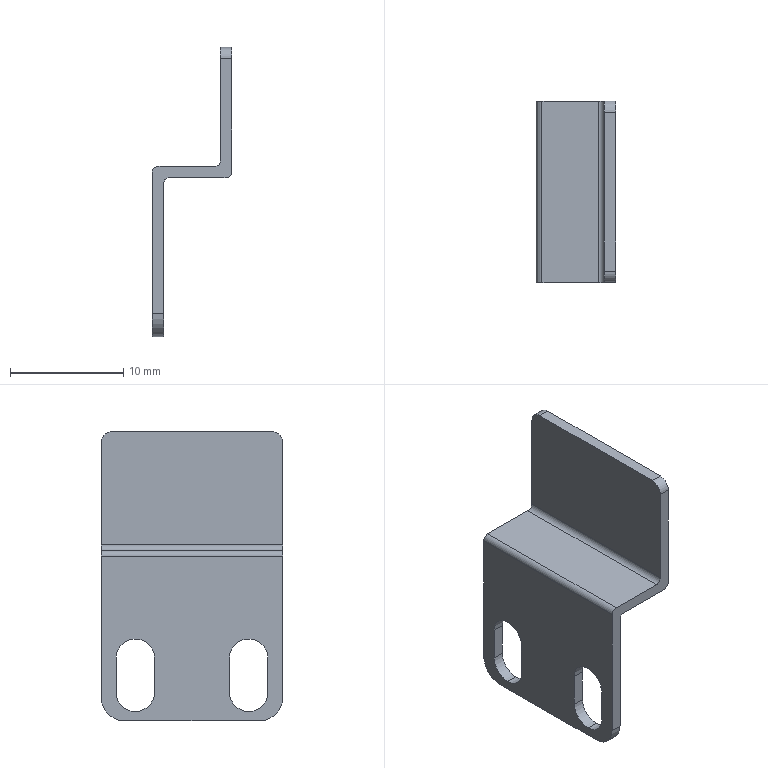Part | SolidWorks | features BaseBody 1 | 1 solid | 28 faces | box 7 x 16 x 25.5 mm | volume 463.296 mm3 | cylinder 14 | plane 14 | commonest cylinder face diameters 3.4 x6 1 x4 2 x2 4 x2
STEP:
#1=CARTESIAN_POINT('',(-4.921,4.7,-20.701));
#2=VERTEX_POINT('',#1);
#3=CARTESIAN_POINT('',(-4.921,3.,-22.401));
#4=VERTEX_POINT('',#3);
#5=CARTESIAN_POINT('',(-4.921,3.,-20.701));
#6=DIRECTION('',(-1.,0.,0.));
#7=DIRECTION('',(0.,0.,-1.));
#8=AXIS2_PLACEMENT_3D('',#5,#6,#7);
#9=CIRCLE('',#8,1.7);
#10=EDGE_CURVE('',#2,#4,#9,.T.);
#11=ORIENTED_EDGE('',*,*,#10,.T.);
#12=CARTESIAN_POINT('',(-3.921,3.,-22.401));
#13=VERTEX_POINT('',#12);
#14=CARTESIAN_POINT('',(-4.921,3.,-22.401));
#15=DIRECTION('',(1.,0.,0.));
#16=VECTOR('',#15,1000.);
#17=LINE('',#14,#16);
#18=EDGE_CURVE('',#4,#13,#17,.T.);
#19=ORIENTED_EDGE('',*,*,#18,.T.);
#20=CARTESIAN_POINT('',(-3.921,4.7,-20.701));
#21=VERTEX_POINT('',#20);
#22=CARTESIAN_POINT('',(-3.921,3.,-20.701));
#23=DIRECTION('',(-1.,0.,0.));
#24=DIRECTION('',(0.,0.,-1.));
#25=AXIS2_PLACEMENT_3D('',#22,#23,#24);
#26=CIRCLE('',#25,1.7);
#27=EDGE_CURVE('',#21,#13,#26,.T.);
#28=ORIENTED_EDGE('',*,*,#27,.F.);
#29=CARTESIAN_POINT('',(-4.921,4.7,-20.701));
#30=DIRECTION('',(1.,0.,0.));
#31=VECTOR('',#30,1000.);
#32=LINE('',#29,#31);
#33=EDGE_CURVE('',#2,#21,#32,.T.);
#34=ORIENTED_EDGE('',*,*,#33,.F.);
#35=EDGE_LOOP('',(#11,#19,#28,#34));
#36=FACE_OUTER_BOUND('',#35,.T.);
#37=CARTESIAN_POINT('',(-4.921,3.,-20.701));
#38=DIRECTION('',(1.,0.,0.));
#39=DIRECTION('',(0.,0.,-1.));
#40=AXIS2_PLACEMENT_3D('',#37,#38,#39);
#41=CYLINDRICAL_SURFACE('',#40,1.7);
#42=ADVANCED_FACE('',(#36),#41,.F.);
#43=CARTESIAN_POINT('',(-4.921,14.7,-20.701));
#44=VERTEX_POINT('',#43);
#45=CARTESIAN_POINT('',(-4.921,13.,-22.401));
#46=VERTEX_POINT('',#45);
#47=CARTESIAN_POINT('',(-4.921,13.,-20.701));
#48=DIRECTION('',(-1.,0.,0.));
#49=DIRECTION('',(0.,0.,-1.));
#50=AXIS2_PLACEMENT_3D('',#47,#48,#49);
#51=CIRCLE('',#50,1.7);
#52=EDGE_CURVE('',#44,#46,#51,.T.);
#53=ORIENTED_EDGE('',*,*,#52,.T.);
#54=CARTESIAN_POINT('',(-3.921,13.,-22.401));
#55=VERTEX_POINT('',#54);
#56=CARTESIAN_POINT('',(-4.921,13.,-22.401));
#57=DIRECTION('',(1.,0.,0.));
#58=VECTOR('',#57,1000.);
#59=LINE('',#56,#58);
#60=EDGE_CURVE('',#46,#55,#59,.T.);
#61=ORIENTED_EDGE('',*,*,#60,.T.);
#62=CARTESIAN_POINT('',(-3.921,14.7,-20.701));
#63=VERTEX_POINT('',#62);
#64=CARTESIAN_POINT('',(-3.921,13.,-20.701));
#65=DIRECTION('',(-1.,0.,0.));
#66=DIRECTION('',(0.,0.,-1.));
#67=AXIS2_PLACEMENT_3D('',#64,#65,#66);
#68=CIRCLE('',#67,1.7);
#69=EDGE_CURVE('',#63,#55,#68,.T.);
#70=ORIENTED_EDGE('',*,*,#69,.F.);
#71=CARTESIAN_POINT('',(-4.921,14.7,-20.701));
#72=DIRECTION('',(1.,0.,0.));
#73=VECTOR('',#72,1000.);
#74=LINE('',#71,#73);
#75=EDGE_CURVE('',#44,#63,#74,.T.);
#76=ORIENTED_EDGE('',*,*,#75,.F.);
#77=EDGE_LOOP('',(#53,#61,#70,#76));
#78=FACE_OUTER_BOUND('',#77,.T.);
#79=CARTESIAN_POINT('',(-4.921,13.,-20.701));
#80=DIRECTION('',(1.,0.,0.));
#81=DIRECTION('',(0.,0.,-1.));
#82=AXIS2_PLACEMENT_3D('',#79,#80,#81);
#83=CYLINDRICAL_SURFACE('',#82,1.7);
#84=ADVANCED_FACE('',(#78),#83,.F.);
#85=CARTESIAN_POINT('',(-4.921,16.,-8.701));
#86=VERTEX_POINT('',#85);
#87=CARTESIAN_POINT('',(-4.921,0.,-8.701));
#88=VERTEX_POINT('',#87);
#89=CARTESIAN_POINT('',(-4.921,16.,-8.701));
#90=DIRECTION('',(0.,-1.,0.));
#91=VECTOR('',#90,1000.);
#92=LINE('',#89,#91);
#93=EDGE_CURVE('',#86,#88,#92,.T.);
#94=ORIENTED_EDGE('',*,*,#93,.F.);
#95=CARTESIAN_POINT('',(-4.921,16.,-21.201));
#96=VERTEX_POINT('',#95);
#97=CARTESIAN_POINT('',(-4.921,16.,-23.201));
#98=DIRECTION('',(0.,0.,1.));
#99=VECTOR('',#98,1000.);
#100=LINE('',#97,#99);
#101=EDGE_CURVE('',#96,#86,#100,.T.);
#102=ORIENTED_EDGE('',*,*,#101,.F.);
#103=CARTESIAN_POINT('',(-4.921,14.,-23.201));
#104=VERTEX_POINT('',#103);
#105=CARTESIAN_POINT('',(-4.921,14.,-21.201));
#106=DIRECTION('',(1.,0.,0.));
#107=DIRECTION('',(0.,0.,-1.));
#108=AXIS2_PLACEMENT_3D('',#105,#106,#107);
#109=CIRCLE('',#108,2.);
#110=EDGE_CURVE('',#104,#96,#109,.T.);
#111=ORIENTED_EDGE('',*,*,#110,.F.);
#112=CARTESIAN_POINT('',(-4.921,2.,-23.201));
#113=VERTEX_POINT('',#112);
#114=CARTESIAN_POINT('',(-4.921,16.,-23.201));
#115=DIRECTION('',(0.,1.,0.));
#116=VECTOR('',#115,1000.);
#117=LINE('',#114,#116);
#118=EDGE_CURVE('',#113,#104,#117,.T.);
#119=ORIENTED_EDGE('',*,*,#118,.F.);
#120=CARTESIAN_POINT('',(-4.921,0.,-21.201));
#121=VERTEX_POINT('',#120);
#122=CARTESIAN_POINT('',(-4.921,2.,-21.201));
#123=DIRECTION('',(1.,0.,0.));
#124=DIRECTION('',(0.,0.,1.));
#125=AXIS2_PLACEMENT_3D('',#122,#123,#124);
#126=CIRCLE('',#125,2.);
#127=EDGE_CURVE('',#121,#113,#126,.T.);
#128=ORIENTED_EDGE('',*,*,#127,.F.);
#129=CARTESIAN_POINT('',(-4.921,0.,-23.201));
#130=DIRECTION('',(0.,0.,-1.));
#131=VECTOR('',#130,1000.);
#132=LINE('',#129,#131);
#133=EDGE_CURVE('',#88,#121,#132,.T.);
#134=ORIENTED_EDGE('',*,*,#133,.F.);
#135=EDGE_LOOP('',(#94,#102,#111,#119,#128,#134));
#136=FACE_OUTER_BOUND('',#135,.T.);
#137=CARTESIAN_POINT('',(-4.921,1.3,-20.701));
#138=VERTEX_POINT('',#137);
#139=CARTESIAN_POINT('',(-4.921,1.3,-17.701));
#140=VERTEX_POINT('',#139);
#141=CARTESIAN_POINT('',(-4.921,1.3,-23.201));
#142=DIRECTION('',(0.,0.,1.));
#143=VECTOR('',#142,1000.);
#144=LINE('',#141,#143);
#145=EDGE_CURVE('',#138,#140,#144,.T.);
#146=ORIENTED_EDGE('',*,*,#145,.F.);
#147=CARTESIAN_POINT('',(-4.921,3.,-20.701));
#148=DIRECTION('',(-1.,0.,0.));
#149=DIRECTION('',(0.,0.,-1.));
#150=AXIS2_PLACEMENT_3D('',#147,#148,#149);
#151=CIRCLE('',#150,1.7);
#152=EDGE_CURVE('',#4,#138,#151,.T.);
#153=ORIENTED_EDGE('',*,*,#152,.F.);
#154=ORIENTED_EDGE('',*,*,#10,.F.);
#155=CARTESIAN_POINT('',(-4.921,4.7,-17.701));
#156=VERTEX_POINT('',#155);
#157=CARTESIAN_POINT('',(-4.921,4.7,-23.201));
#158=DIRECTION('',(0.,0.,-1.));
#159=VECTOR('',#158,1000.);
#160=LINE('',#157,#159);
#161=EDGE_CURVE('',#156,#2,#160,.T.);
#162=ORIENTED_EDGE('',*,*,#161,.F.);
#163=CARTESIAN_POINT('',(-4.921,3.,-17.701));
#164=DIRECTION('',(-1.,0.,0.));
#165=DIRECTION('',(0.,0.,-1.));
#166=AXIS2_PLACEMENT_3D('',#163,#164,#165);
#167=CIRCLE('',#166,1.7);
#168=EDGE_CURVE('',#140,#156,#167,.T.);
#169=ORIENTED_EDGE('',*,*,#168,.F.);
#170=EDGE_LOOP('',(#146,#153,#154,#162,#169));
#171=FACE_BOUND('',#170,.T.);
#172=CARTESIAN_POINT('',(-4.921,11.3,-20.701));
#173=VERTEX_POINT('',#172);
#174=CARTESIAN_POINT('',(-4.921,11.3,-17.701));
#175=VERTEX_POINT('',#174);
#176=CARTESIAN_POINT('',(-4.921,11.3,-23.201));
#177=DIRECTION('',(0.,0.,1.));
#178=VECTOR('',#177,1000.);
#179=LINE('',#176,#178);
#180=EDGE_CURVE('',#173,#175,#179,.T.);
#181=ORIENTED_EDGE('',*,*,#180,.F.);
#182=CARTESIAN_POINT('',(-4.921,13.,-20.701));
#183=DIRECTION('',(-1.,0.,0.));
#184=DIRECTION('',(0.,0.,-1.));
#185=AXIS2_PLACEMENT_3D('',#182,#183,#184);
#186=CIRCLE('',#185,1.7);
#187=EDGE_CURVE('',#46,#173,#186,.T.);
#188=ORIENTED_EDGE('',*,*,#187,.F.);
#189=ORIENTED_EDGE('',*,*,#52,.F.);
#190=CARTESIAN_POINT('',(-4.921,14.7,-17.701));
#191=VERTEX_POINT('',#190);
#192=CARTESIAN_POINT('',(-4.921,14.7,-23.201));
#193=DIRECTION('',(0.,0.,-1.));
#194=VECTOR('',#193,1000.);
#195=LINE('',#192,#194);
#196=EDGE_CURVE('',#191,#44,#195,.T.);
#197=ORIENTED_EDGE('',*,*,#196,.F.);
#198=CARTESIAN_POINT('',(-4.921,13.,-17.701));
#199=DIRECTION('',(-1.,0.,0.));
#200=DIRECTION('',(0.,0.,-1.));
#201=AXIS2_PLACEMENT_3D('',#198,#199,#200);
#202=CIRCLE('',#201,1.7);
#203=EDGE_CURVE('',#175,#191,#202,.T.);
#204=ORIENTED_EDGE('',*,*,#203,.F.);
#205=EDGE_LOOP('',(#181,#188,#189,#197,#204));
#206=FACE_BOUND('',#205,.T.);
#207=CARTESIAN_POINT('',(-4.921,16.,-23.201));
#208=DIRECTION('',(1.,0.,0.));
#209=DIRECTION('',(0.,0.,-1.));
#210=AXIS2_PLACEMENT_3D('',#207,#208,#209);
#211=PLANE('',#210);
#212=ADVANCED_FACE('',(#136,#171,#206),#211,.F.);
#213=CARTESIAN_POINT('',(1.079,0.,1.299));
#214=VERTEX_POINT('',#213);
#215=CARTESIAN_POINT('',(2.079,0.,1.299));
#216=VERTEX_POINT('',#215);
#217=CARTESIAN_POINT('',(0.,0.,1.299));
#218=DIRECTION('',(1.,0.,0.));
#219=VECTOR('',#218,1000.);
#220=LINE('',#217,#219);
#221=EDGE_CURVE('',#214,#216,#220,.T.);
#222=ORIENTED_EDGE('',*,*,#221,.F.);
#223=CARTESIAN_POINT('',(1.079,0.,-7.701));
#224=VERTEX_POINT('',#223);
#225=CARTESIAN_POINT('',(1.079,0.,0.));
#226=DIRECTION('',(0.,0.,1.));
#227=VECTOR('',#226,1000.);
#228=LINE('',#225,#227);
#229=EDGE_CURVE('',#224,#214,#228,.T.);
#230=ORIENTED_EDGE('',*,*,#229,.F.);
#231=CARTESIAN_POINT('',(0.5794,0.,-8.201));
#232=VERTEX_POINT('',#231);
#233=CARTESIAN_POINT('',(0.5794,0.,-7.701));
#234=DIRECTION('',(0.,-1.,0.));
#235=DIRECTION('',(0.,0.,1.));
#236=AXIS2_PLACEMENT_3D('',#233,#234,#235);
#237=CIRCLE('',#236,0.5);
#238=EDGE_CURVE('',#232,#224,#237,.T.);
#239=ORIENTED_EDGE('',*,*,#238,.F.);
#240=CARTESIAN_POINT('',(-4.421,0.,-8.201));
#241=VERTEX_POINT('',#240);
#242=CARTESIAN_POINT('',(0.,0.,-8.201));
#243=DIRECTION('',(1.,0.,0.));
#244=VECTOR('',#243,1000.);
#245=LINE('',#242,#244);
#246=EDGE_CURVE('',#241,#232,#245,.T.);
#247=ORIENTED_EDGE('',*,*,#246,.F.);
#248=CARTESIAN_POINT('',(-4.421,0.,-8.701));
#249=DIRECTION('',(0.,1.,0.));
#250=DIRECTION('',(0.,0.,-1.));
#251=AXIS2_PLACEMENT_3D('',#248,#249,#250);
#252=CIRCLE('',#251,0.5);
#253=EDGE_CURVE('',#88,#241,#252,.T.);
#254=ORIENTED_EDGE('',*,*,#253,.F.);
#255=ORIENTED_EDGE('',*,*,#133,.T.);
#256=CARTESIAN_POINT('',(-3.921,0.,-21.201));
#257=VERTEX_POINT('',#256);
#258=CARTESIAN_POINT('',(0.,0.,-21.201));
#259=DIRECTION('',(-1.,0.,0.));
#260=VECTOR('',#259,1000.);
#261=LINE('',#258,#260);
#262=EDGE_CURVE('',#257,#121,#261,.T.);
#263=ORIENTED_EDGE('',*,*,#262,.F.);
#264=CARTESIAN_POINT('',(-3.921,0.,-9.701));
#265=VERTEX_POINT('',#264);
#266=CARTESIAN_POINT('',(-3.921,0.,0.));
#267=DIRECTION('',(0.,0.,-1.));
#268=VECTOR('',#267,1000.);
#269=LINE('',#266,#268);
#270=EDGE_CURVE('',#265,#257,#269,.T.);
#271=ORIENTED_EDGE('',*,*,#270,.F.);
#272=CARTESIAN_POINT('',(-3.421,0.,-9.201));
#273=VERTEX_POINT('',#272);
#274=CARTESIAN_POINT('',(-3.421,0.,-9.701));
#275=DIRECTION('',(0.,-1.,0.));
#276=DIRECTION('',(0.,0.,1.));
#277=AXIS2_PLACEMENT_3D('',#274,#275,#276);
#278=CIRCLE('',#277,0.5);
#279=EDGE_CURVE('',#273,#265,#278,.T.);
#280=ORIENTED_EDGE('',*,*,#279,.F.);
#281=CARTESIAN_POINT('',(1.579,0.,-9.201));
#282=VERTEX_POINT('',#281);
#283=CARTESIAN_POINT('',(0.,0.,-9.201));
#284=DIRECTION('',(-1.,0.,0.));
#285=VECTOR('',#284,1000.);
#286=LINE('',#283,#285);
#287=EDGE_CURVE('',#282,#273,#286,.T.);
#288=ORIENTED_EDGE('',*,*,#287,.F.);
#289=CARTESIAN_POINT('',(2.079,0.,-8.701));
#290=VERTEX_POINT('',#289);
#291=CARTESIAN_POINT('',(1.579,0.,-8.701));
#292=DIRECTION('',(0.,1.,0.));
#293=DIRECTION('',(0.,0.,-1.));
#294=AXIS2_PLACEMENT_3D('',#291,#292,#293);
#295=CIRCLE('',#294,0.5);
#296=EDGE_CURVE('',#290,#282,#295,.T.);
#297=ORIENTED_EDGE('',*,*,#296,.F.);
#298=CARTESIAN_POINT('',(2.079,0.,0.));
#299=DIRECTION('',(0.,0.,-1.));
#300=VECTOR('',#299,1000.);
#301=LINE('',#298,#300);
#302=EDGE_CURVE('',#216,#290,#301,.T.);
#303=ORIENTED_EDGE('',*,*,#302,.F.);
#304=EDGE_LOOP('',(#222,#230,#239,#247,#254,#255,#263,#271,#280,#288,#297,#303));
#305=FACE_OUTER_BOUND('',#304,.T.);
#306=CARTESIAN_POINT('',(0.,0.,0.));
#307=DIRECTION('',(0.,1.,0.));
#308=DIRECTION('',(0.,0.,1.));
#309=AXIS2_PLACEMENT_3D('',#306,#307,#308);
#310=PLANE('',#309);
#311=ADVANCED_FACE('',(#305),#310,.F.);
#312=ORIENTED_EDGE('',*,*,#253,.T.);
#313=CARTESIAN_POINT('',(-4.421,16.,-8.201));
#314=VERTEX_POINT('',#313);
#315=CARTESIAN_POINT('',(-4.421,16.,-8.201));
#316=DIRECTION('',(0.,1.,0.));
#317=VECTOR('',#316,1000.);
#318=LINE('',#315,#317);
#319=EDGE_CURVE('',#241,#314,#318,.T.);
#320=ORIENTED_EDGE('',*,*,#319,.T.);
#321=CARTESIAN_POINT('',(-4.421,16.,-8.701));
#322=DIRECTION('',(0.,-1.,0.));
#323=DIRECTION('',(0.,0.,-1.));
#324=AXIS2_PLACEMENT_3D('',#321,#322,#323);
#325=CIRCLE('',#324,0.5);
#326=EDGE_CURVE('',#314,#86,#325,.T.);
#327=ORIENTED_EDGE('',*,*,#326,.T.);
#328=ORIENTED_EDGE('',*,*,#93,.T.);
#329=EDGE_LOOP('',(#312,#320,#327,#328));
#330=FACE_OUTER_BOUND('',#329,.T.);
#331=CARTESIAN_POINT('',(-4.421,16.,-8.701));
#332=DIRECTION('',(0.,-1.,0.));
#333=DIRECTION('',(0.,0.,-1.));
#334=AXIS2_PLACEMENT_3D('',#331,#332,#333);
#335=CYLINDRICAL_SURFACE('',#334,0.5);
#336=ADVANCED_FACE('',(#330),#335,.T.);
#337=CARTESIAN_POINT('',(0.5794,16.,-8.201));
#338=VERTEX_POINT('',#337);
#339=CARTESIAN_POINT('',(0.,16.,-8.201));
#340=DIRECTION('',(1.,0.,0.));
#341=VECTOR('',#340,1000.);
#342=LINE('',#339,#341);
#343=EDGE_CURVE('',#314,#338,#342,.T.);
#344=ORIENTED_EDGE('',*,*,#343,.T.);
#345=CARTESIAN_POINT('',(1.079,16.,-7.701));
#346=VERTEX_POINT('',#345);
#347=CARTESIAN_POINT('',(0.5794,16.,-7.701));
#348=DIRECTION('',(0.,-1.,0.));
#349=DIRECTION('',(0.,0.,1.));
#350=AXIS2_PLACEMENT_3D('',#347,#348,#349);
#351=CIRCLE('',#350,0.5);
#352=EDGE_CURVE('',#338,#346,#351,.T.);
#353=ORIENTED_EDGE('',*,*,#352,.T.);
#354=CARTESIAN_POINT('',(1.079,16.,1.299));
#355=VERTEX_POINT('',#354);
#356=CARTESIAN_POINT('',(1.079,16.,0.));
#357=DIRECTION('',(0.,0.,1.));
#358=VECTOR('',#357,1000.);
#359=LINE('',#356,#358);
#360=EDGE_CURVE('',#346,#355,#359,.T.);
#361=ORIENTED_EDGE('',*,*,#360,.T.);
#362=CARTESIAN_POINT('',(2.079,16.,1.299));
#363=VERTEX_POINT('',#362);
#364=CARTESIAN_POINT('',(0.,16.,1.299));
#365=DIRECTION('',(1.,0.,0.));
#366=VECTOR('',#365,1000.);
#367=LINE('',#364,#366);
#368=EDGE_CURVE('',#355,#363,#367,.T.);
#369=ORIENTED_EDGE('',*,*,#368,.T.);
#370=CARTESIAN_POINT('',(2.079,16.,-8.701));
#371=VERTEX_POINT('',#370);
#372=CARTESIAN_POINT('',(2.079,16.,0.));
#373=DIRECTION('',(0.,0.,-1.));
#374=VECTOR('',#373,1000.);
#375=LINE('',#372,#374);
#376=EDGE_CURVE('',#363,#371,#375,.T.);
#377=ORIENTED_EDGE('',*,*,#376,.T.);
#378=CARTESIAN_POINT('',(1.579,16.,-9.201));
#379=VERTEX_POINT('',#378);
#380=CARTESIAN_POINT('',(1.579,16.,-8.701));
#381=DIRECTION('',(0.,1.,0.));
#382=DIRECTION('',(0.,0.,-1.));
#383=AXIS2_PLACEMENT_3D('',#380,#381,#382);
#384=CIRCLE('',#383,0.5);
#385=EDGE_CURVE('',#371,#379,#384,.T.);
#386=ORIENTED_EDGE('',*,*,#385,.T.);
#387=CARTESIAN_POINT('',(-3.421,16.,-9.201));
#388=VERTEX_POINT('',#387);
#389=CARTESIAN_POINT('',(0.,16.,-9.201));
#390=DIRECTION('',(-1.,0.,0.));
#391=VECTOR('',#390,1000.);
#392=LINE('',#389,#391);
#393=EDGE_CURVE('',#379,#388,#392,.T.);
#394=ORIENTED_EDGE('',*,*,#393,.T.);
#395=CARTESIAN_POINT('',(-3.921,16.,-9.701));
#396=VERTEX_POINT('',#395);
#397=CARTESIAN_POINT('',(-3.421,16.,-9.701));
#398=DIRECTION('',(0.,-1.,0.));
#399=DIRECTION('',(0.,0.,1.));
#400=AXIS2_PLACEMENT_3D('',#397,#398,#399);
#401=CIRCLE('',#400,0.5);
#402=EDGE_CURVE('',#388,#396,#401,.T.);
#403=ORIENTED_EDGE('',*,*,#402,.T.);
#404=CARTESIAN_POINT('',(-3.921,16.,-21.201));
#405=VERTEX_POINT('',#404);
#406=CARTESIAN_POINT('',(-3.921,16.,0.));
#407=DIRECTION('',(0.,0.,-1.));
#408=VECTOR('',#407,1000.);
#409=LINE('',#406,#408);
#410=EDGE_CURVE('',#396,#405,#409,.T.);
#411=ORIENTED_EDGE('',*,*,#410,.T.);
#412=CARTESIAN_POINT('',(0.,16.,-21.201));
#413=DIRECTION('',(-1.,0.,0.));
#414=VECTOR('',#413,1000.);
#415=LINE('',#412,#414);
#416=EDGE_CURVE('',#405,#96,#415,.T.);
#417=ORIENTED_EDGE('',*,*,#416,.T.);
#418=ORIENTED_EDGE('',*,*,#101,.T.);
#419=ORIENTED_EDGE('',*,*,#326,.F.);
#420=EDGE_LOOP('',(#344,#353,#361,#369,#377,#386,#394,#403,#411,#417,#418,#419));
#421=FACE_OUTER_BOUND('',#420,.T.);
#422=CARTESIAN_POINT('',(0.,16.,0.));
#423=DIRECTION('',(0.,1.,0.));
#424=DIRECTION('',(0.,0.,1.));
#425=AXIS2_PLACEMENT_3D('',#422,#423,#424);
#426=PLANE('',#425);
#427=ADVANCED_FACE('',(#421),#426,.T.);
#428=ORIENTED_EDGE('',*,*,#110,.T.);
#429=ORIENTED_EDGE('',*,*,#416,.F.);
#430=CARTESIAN_POINT('',(-3.921,14.,-23.201));
#431=VERTEX_POINT('',#430);
#432=CARTESIAN_POINT('',(-3.921,14.,-21.201));
#433=DIRECTION('',(-1.,0.,0.));
#434=DIRECTION('',(0.,0.,-1.));
#435=AXIS2_PLACEMENT_3D('',#432,#433,#434);
#436=CIRCLE('',#435,2.);
#437=EDGE_CURVE('',#405,#431,#436,.T.);
#438=ORIENTED_EDGE('',*,*,#437,.T.);
#439=CARTESIAN_POINT('',(0.,14.,-23.201));
#440=DIRECTION('',(-1.,0.,0.));
#441=VECTOR('',#440,1000.);
#442=LINE('',#439,#441);
#443=EDGE_CURVE('',#431,#104,#442,.T.);
#444=ORIENTED_EDGE('',*,*,#443,.T.);
#445=EDGE_LOOP('',(#428,#429,#438,#444));
#446=FACE_OUTER_BOUND('',#445,.T.);
#447=CARTESIAN_POINT('',(0.,14.,-21.201));
#448=DIRECTION('',(1.,0.,0.));
#449=DIRECTION('',(0.,0.,-1.));
#450=AXIS2_PLACEMENT_3D('',#447,#448,#449);
#451=CYLINDRICAL_SURFACE('',#450,2.);
#452=ADVANCED_FACE('',(#446),#451,.T.);
#453=ORIENTED_EDGE('',*,*,#443,.F.);
#454=CARTESIAN_POINT('',(-3.921,2.,-23.201));
#455=VERTEX_POINT('',#454);
#456=CARTESIAN_POINT('',(-3.921,16.,-23.201));
#457=DIRECTION('',(0.,1.,0.));
#458=VECTOR('',#457,1000.);
#459=LINE('',#456,#458);
#460=EDGE_CURVE('',#455,#431,#459,.T.);
#461=ORIENTED_EDGE('',*,*,#460,.F.);
#462=CARTESIAN_POINT('',(-4.921,2.,-23.201));
#463=DIRECTION('',(1.,0.,0.));
#464=VECTOR('',#463,1000.);
#465=LINE('',#462,#464);
#466=EDGE_CURVE('',#113,#455,#465,.T.);
#467=ORIENTED_EDGE('',*,*,#466,.F.);
#468=ORIENTED_EDGE('',*,*,#118,.T.);
#469=EDGE_LOOP('',(#453,#461,#467,#468));
#470=FACE_OUTER_BOUND('',#469,.T.);
#471=CARTESIAN_POINT('',(-4.921,16.,-23.201));
#472=DIRECTION('',(0.,0.,1.));
#473=DIRECTION('',(1.,0.,0.));
#474=AXIS2_PLACEMENT_3D('',#471,#472,#473);
#475=PLANE('',#474);
#476=ADVANCED_FACE('',(#470),#475,.F.);
#477=ORIENTED_EDGE('',*,*,#127,.T.);
#478=ORIENTED_EDGE('',*,*,#466,.T.);
#479=CARTESIAN_POINT('',(-3.921,2.,-21.201));
#480=DIRECTION('',(-1.,0.,0.));
#481=DIRECTION('',(0.,0.,1.));
#482=AXIS2_PLACEMENT_3D('',#479,#480,#481);
#483=CIRCLE('',#482,2.);
#484=EDGE_CURVE('',#455,#257,#483,.T.);
#485=ORIENTED_EDGE('',*,*,#484,.T.);
#486=ORIENTED_EDGE('',*,*,#262,.T.);
#487=EDGE_LOOP('',(#477,#478,#485,#486));
#488=FACE_OUTER_BOUND('',#487,.T.);
#489=CARTESIAN_POINT('',(-4.921,2.,-21.201));
#490=DIRECTION('',(-1.,0.,0.));
#491=DIRECTION('',(0.,0.,1.));
#492=AXIS2_PLACEMENT_3D('',#489,#490,#491);
#493=CYLINDRICAL_SURFACE('',#492,2.);
#494=ADVANCED_FACE('',(#488),#493,.T.);
#495=CARTESIAN_POINT('',(-3.921,1.3,-17.701));
#496=VERTEX_POINT('',#495);
#497=CARTESIAN_POINT('',(-4.921,1.3,-17.701));
#498=DIRECTION('',(1.,0.,0.));
#499=VECTOR('',#498,1000.);
#500=LINE('',#497,#499);
#501=EDGE_CURVE('',#140,#496,#500,.T.);
#502=ORIENTED_EDGE('',*,*,#501,.F.);
#503=ORIENTED_EDGE('',*,*,#168,.T.);
#504=CARTESIAN_POINT('',(-3.921,4.7,-17.701));
#505=VERTEX_POINT('',#504);
#506=CARTESIAN_POINT('',(-4.921,4.7,-17.701));
#507=DIRECTION('',(-1.,0.,0.));
#508=VECTOR('',#507,1000.);
#509=LINE('',#506,#508);
#510=EDGE_CURVE('',#505,#156,#509,.T.);
#511=ORIENTED_EDGE('',*,*,#510,.F.);
#512=CARTESIAN_POINT('',(-3.921,3.,-17.701));
#513=DIRECTION('',(-1.,0.,0.));
#514=DIRECTION('',(0.,0.,-1.));
#515=AXIS2_PLACEMENT_3D('',#512,#513,#514);
#516=CIRCLE('',#515,1.7);
#517=EDGE_CURVE('',#496,#505,#516,.T.);
#518=ORIENTED_EDGE('',*,*,#517,.F.);
#519=EDGE_LOOP('',(#502,#503,#511,#518));
#520=FACE_OUTER_BOUND('',#519,.T.);
#521=CARTESIAN_POINT('',(-4.921,3.,-17.701));
#522=DIRECTION('',(1.,0.,0.));
#523=DIRECTION('',(0.,0.,-1.));
#524=AXIS2_PLACEMENT_3D('',#521,#522,#523);
#525=CYLINDRICAL_SURFACE('',#524,1.7);
#526=ADVANCED_FACE('',(#520),#525,.F.);
#527=CARTESIAN_POINT('',(-3.921,1.3,-20.701));
#528=VERTEX_POINT('',#527);
#529=CARTESIAN_POINT('',(-4.921,1.3,-20.701));
#530=DIRECTION('',(1.,0.,0.));
#531=VECTOR('',#530,1000.);
#532=LINE('',#529,#531);
#533=EDGE_CURVE('',#138,#528,#532,.T.);
#534=ORIENTED_EDGE('',*,*,#533,.F.);
#535=ORIENTED_EDGE('',*,*,#145,.T.);
#536=ORIENTED_EDGE('',*,*,#501,.T.);
#537=CARTESIAN_POINT('',(-3.921,1.3,-20.701));
#538=DIRECTION('',(0.,0.,1.));
#539=VECTOR('',#538,1000.);
#540=LINE('',#537,#539);
#541=EDGE_CURVE('',#528,#496,#540,.T.);
#542=ORIENTED_EDGE('',*,*,#541,.F.);
#543=EDGE_LOOP('',(#534,#535,#536,#542));
#544=FACE_OUTER_BOUND('',#543,.T.);
#545=CARTESIAN_POINT('',(-4.921,1.3,-20.701));
#546=DIRECTION('',(0.,-1.,0.));
#547=DIRECTION('',(0.,0.,-1.));
#548=AXIS2_PLACEMENT_3D('',#545,#546,#547);
#549=PLANE('',#548);
#550=ADVANCED_FACE('',(#544),#549,.F.);
#551=ORIENTED_EDGE('',*,*,#18,.F.);
#552=ORIENTED_EDGE('',*,*,#152,.T.);
#553=ORIENTED_EDGE('',*,*,#533,.T.);
#554=CARTESIAN_POINT('',(-3.921,3.,-20.701));
#555=DIRECTION('',(-1.,0.,0.));
#556=DIRECTION('',(0.,0.,-1.));
#557=AXIS2_PLACEMENT_3D('',#554,#555,#556);
#558=CIRCLE('',#557,1.7);
#559=EDGE_CURVE('',#13,#528,#558,.T.);
#560=ORIENTED_EDGE('',*,*,#559,.F.);
#561=EDGE_LOOP('',(#551,#552,#553,#560));
#562=FACE_OUTER_BOUND('',#561,.T.);
#563=CARTESIAN_POINT('',(-4.921,3.,-20.701));
#564=DIRECTION('',(1.,0.,0.));
#565=DIRECTION('',(0.,0.,-1.));
#566=AXIS2_PLACEMENT_3D('',#563,#564,#565);
#567=CYLINDRICAL_SURFACE('',#566,1.7);
#568=ADVANCED_FACE('',(#562),#567,.F.);
#569=ORIENTED_EDGE('',*,*,#510,.T.);
#570=ORIENTED_EDGE('',*,*,#161,.T.);
#571=ORIENTED_EDGE('',*,*,#33,.T.);
#572=CARTESIAN_POINT('',(-3.921,4.7,-20.701));
#573=DIRECTION('',(0.,0.,-1.));
#574=VECTOR('',#573,1000.);
#575=LINE('',#572,#574);
#576=EDGE_CURVE('',#505,#21,#575,.T.);
#577=ORIENTED_EDGE('',*,*,#576,.F.);
#578=EDGE_LOOP('',(#569,#570,#571,#577));
#579=FACE_OUTER_BOUND('',#578,.T.);
#580=CARTESIAN_POINT('',(-4.921,4.7,-20.701));
#581=DIRECTION('',(0.,1.,0.));
#582=DIRECTION('',(0.,0.,1.));
#583=AXIS2_PLACEMENT_3D('',#580,#581,#582);
#584=PLANE('',#583);
#585=ADVANCED_FACE('',(#579),#584,.F.);
#586=CARTESIAN_POINT('',(-3.921,11.3,-17.701));
#587=VERTEX_POINT('',#586);
#588=CARTESIAN_POINT('',(-4.921,11.3,-17.701));
#589=DIRECTION('',(1.,0.,0.));
#590=VECTOR('',#589,1000.);
#591=LINE('',#588,#590);
#592=EDGE_CURVE('',#175,#587,#591,.T.);
#593=ORIENTED_EDGE('',*,*,#592,.F.);
#594=ORIENTED_EDGE('',*,*,#203,.T.);
#595=CARTESIAN_POINT('',(-3.921,14.7,-17.701));
#596=VERTEX_POINT('',#595);
#597=CARTESIAN_POINT('',(-4.921,14.7,-17.701));
#598=DIRECTION('',(-1.,0.,0.));
#599=VECTOR('',#598,1000.);
#600=LINE('',#597,#599);
#601=EDGE_CURVE('',#596,#191,#600,.T.);
#602=ORIENTED_EDGE('',*,*,#601,.F.);
#603=CARTESIAN_POINT('',(-3.921,13.,-17.701));
#604=DIRECTION('',(-1.,0.,0.));
#605=DIRECTION('',(0.,0.,-1.));
#606=AXIS2_PLACEMENT_3D('',#603,#604,#605);
#607=CIRCLE('',#606,1.7);
#608=EDGE_CURVE('',#587,#596,#607,.T.);
#609=ORIENTED_EDGE('',*,*,#608,.F.);
#610=EDGE_LOOP('',(#593,#594,#602,#609));
#611=FACE_OUTER_BOUND('',#610,.T.);
#612=CARTESIAN_POINT('',(-4.921,13.,-17.701));
#613=DIRECTION('',(1.,0.,0.));
#614=DIRECTION('',(0.,0.,-1.));
#615=AXIS2_PLACEMENT_3D('',#612,#613,#614);
#616=CYLINDRICAL_SURFACE('',#615,1.7);
#617=ADVANCED_FACE('',(#611),#616,.F.);
#618=CARTESIAN_POINT('',(-3.921,11.3,-20.701));
#619=VERTEX_POINT('',#618);
#620=CARTESIAN_POINT('',(-4.921,11.3,-20.701));
#621=DIRECTION('',(1.,0.,0.));
#622=VECTOR('',#621,1000.);
#623=LINE('',#620,#622);
#624=EDGE_CURVE('',#173,#619,#623,.T.);
#625=ORIENTED_EDGE('',*,*,#624,.F.);
#626=ORIENTED_EDGE('',*,*,#180,.T.);
#627=ORIENTED_EDGE('',*,*,#592,.T.);
#628=CARTESIAN_POINT('',(-3.921,11.3,-20.701));
#629=DIRECTION('',(0.,0.,1.));
#630=VECTOR('',#629,1000.);
#631=LINE('',#628,#630);
#632=EDGE_CURVE('',#619,#587,#631,.T.);
#633=ORIENTED_EDGE('',*,*,#632,.F.);
#634=EDGE_LOOP('',(#625,#626,#627,#633));
#635=FACE_OUTER_BOUND('',#634,.T.);
#636=CARTESIAN_POINT('',(-4.921,11.3,-20.701));
#637=DIRECTION('',(0.,-1.,0.));
#638=DIRECTION('',(0.,0.,-1.));
#639=AXIS2_PLACEMENT_3D('',#636,#637,#638);
#640=PLANE('',#639);
#641=ADVANCED_FACE('',(#635),#640,.F.);
#642=ORIENTED_EDGE('',*,*,#60,.F.);
#643=ORIENTED_EDGE('',*,*,#187,.T.);
#644=ORIENTED_EDGE('',*,*,#624,.T.);
#645=CARTESIAN_POINT('',(-3.921,13.,-20.701));
#646=DIRECTION('',(-1.,0.,0.));
#647=DIRECTION('',(0.,0.,-1.));
#648=AXIS2_PLACEMENT_3D('',#645,#646,#647);
#649=CIRCLE('',#648,1.7);
#650=EDGE_CURVE('',#55,#619,#649,.T.);
#651=ORIENTED_EDGE('',*,*,#650,.F.);
#652=EDGE_LOOP('',(#642,#643,#644,#651));
#653=FACE_OUTER_BOUND('',#652,.T.);
#654=CARTESIAN_POINT('',(-4.921,13.,-20.701));
#655=DIRECTION('',(1.,0.,0.));
#656=DIRECTION('',(0.,0.,-1.));
#657=AXIS2_PLACEMENT_3D('',#654,#655,#656);
#658=CYLINDRICAL_SURFACE('',#657,1.7);
#659=ADVANCED_FACE('',(#653),#658,.F.);
#660=ORIENTED_EDGE('',*,*,#601,.T.);
#661=ORIENTED_EDGE('',*,*,#196,.T.);
#662=ORIENTED_EDGE('',*,*,#75,.T.);
#663=CARTESIAN_POINT('',(-3.921,14.7,-20.701));
#664=DIRECTION('',(0.,0.,-1.));
#665=VECTOR('',#664,1000.);
#666=LINE('',#663,#665);
#667=EDGE_CURVE('',#596,#63,#666,.T.);
#668=ORIENTED_EDGE('',*,*,#667,.F.);
#669=EDGE_LOOP('',(#660,#661,#662,#668));
#670=FACE_OUTER_BOUND('',#669,.T.);
#671=CARTESIAN_POINT('',(-4.921,14.7,-20.701));
#672=DIRECTION('',(0.,1.,0.));
#673=DIRECTION('',(0.,0.,1.));
#674=AXIS2_PLACEMENT_3D('',#671,#672,#673);
#675=PLANE('',#674);
#676=ADVANCED_FACE('',(#670),#675,.F.);
#677=CARTESIAN_POINT('',(2.079,1.,2.299));
#678=VERTEX_POINT('',#677);
#679=CARTESIAN_POINT('',(2.079,1.,1.299));
#680=DIRECTION('',(-1.,0.,0.));
#681=DIRECTION('',(0.,0.,-1.));
#682=AXIS2_PLACEMENT_3D('',#679,#680,#681);
#683=CIRCLE('',#682,1.);
#684=EDGE_CURVE('',#216,#678,#683,.T.);
#685=ORIENTED_EDGE('',*,*,#684,.F.);
#686=ORIENTED_EDGE('',*,*,#302,.T.);
#687=CARTESIAN_POINT('',(2.079,16.,-8.701));
#688=DIRECTION('',(0.,-1.,0.));
#689=VECTOR('',#688,1000.);
#690=LINE('',#687,#689);
#691=EDGE_CURVE('',#371,#290,#690,.T.);
#692=ORIENTED_EDGE('',*,*,#691,.F.);
#693=ORIENTED_EDGE('',*,*,#376,.F.);
#694=CARTESIAN_POINT('',(2.079,15.,2.299));
#695=VERTEX_POINT('',#694);
#696=CARTESIAN_POINT('',(2.079,15.,1.299));
#697=DIRECTION('',(-1.,0.,0.));
#698=DIRECTION('',(0.,0.,1.));
#699=AXIS2_PLACEMENT_3D('',#696,#697,#698);
#700=CIRCLE('',#699,1.);
#701=EDGE_CURVE('',#695,#363,#700,.T.);
#702=ORIENTED_EDGE('',*,*,#701,.F.);
#703=CARTESIAN_POINT('',(2.079,16.,2.299));
#704=DIRECTION('',(0.,1.,0.));
#705=VECTOR('',#704,1000.);
#706=LINE('',#703,#705);
#707=EDGE_CURVE('',#678,#695,#706,.T.);
#708=ORIENTED_EDGE('',*,*,#707,.F.);
#709=EDGE_LOOP('',(#685,#686,#692,#693,#702,#708));
#710=FACE_OUTER_BOUND('',#709,.T.);
#711=CARTESIAN_POINT('',(2.079,16.,-9.201));
#712=DIRECTION('',(-1.,0.,0.));
#713=DIRECTION('',(0.,0.,1.));
#714=AXIS2_PLACEMENT_3D('',#711,#712,#713);
#715=PLANE('',#714);
#716=ADVANCED_FACE('',(#710),#715,.F.);
#717=ORIENTED_EDGE('',*,*,#684,.T.);
#718=CARTESIAN_POINT('',(1.079,1.,2.299));
#719=VERTEX_POINT('',#718);
#720=CARTESIAN_POINT('',(2.079,1.,2.299));
#721=DIRECTION('',(-1.,0.,0.));
#722=VECTOR('',#721,1000.);
#723=LINE('',#720,#722);
#724=EDGE_CURVE('',#678,#719,#723,.T.);
#725=ORIENTED_EDGE('',*,*,#724,.T.);
#726=CARTESIAN_POINT('',(1.079,1.,1.299));
#727=DIRECTION('',(1.,0.,0.));
#728=DIRECTION('',(0.,0.,-1.));
#729=AXIS2_PLACEMENT_3D('',#726,#727,#728);
#730=CIRCLE('',#729,1.);
#731=EDGE_CURVE('',#719,#214,#730,.T.);
#732=ORIENTED_EDGE('',*,*,#731,.T.);
#733=ORIENTED_EDGE('',*,*,#221,.T.);
#734=EDGE_LOOP('',(#717,#725,#732,#733));
#735=FACE_OUTER_BOUND('',#734,.T.);
#736=CARTESIAN_POINT('',(2.079,1.,1.299));
#737=DIRECTION('',(1.,0.,0.));
#738=DIRECTION('',(0.,0.,-1.));
#739=AXIS2_PLACEMENT_3D('',#736,#737,#738);
#740=CYLINDRICAL_SURFACE('',#739,1.);
#741=ADVANCED_FACE('',(#735),#740,.T.);
#742=ORIENTED_EDGE('',*,*,#731,.F.);
#743=CARTESIAN_POINT('',(1.079,15.,2.299));
#744=VERTEX_POINT('',#743);
#745=CARTESIAN_POINT('',(1.079,16.,2.299));
#746=DIRECTION('',(0.,-1.,0.));
#747=VECTOR('',#746,1000.);
#748=LINE('',#745,#747);
#749=EDGE_CURVE('',#744,#719,#748,.T.);
#750=ORIENTED_EDGE('',*,*,#749,.F.);
#751=CARTESIAN_POINT('',(1.079,15.,1.299));
#752=DIRECTION('',(1.,0.,0.));
#753=DIRECTION('',(0.,0.,1.));
#754=AXIS2_PLACEMENT_3D('',#751,#752,#753);
#755=CIRCLE('',#754,1.);
#756=EDGE_CURVE('',#355,#744,#755,.T.);
#757=ORIENTED_EDGE('',*,*,#756,.F.);
#758=ORIENTED_EDGE('',*,*,#360,.F.);
#759=CARTESIAN_POINT('',(1.079,16.,-7.701));
#760=DIRECTION('',(0.,1.,0.));
#761=VECTOR('',#760,1000.);
#762=LINE('',#759,#761);
#763=EDGE_CURVE('',#224,#346,#762,.T.);
#764=ORIENTED_EDGE('',*,*,#763,.F.);
#765=ORIENTED_EDGE('',*,*,#229,.T.);
#766=EDGE_LOOP('',(#742,#750,#757,#758,#764,#765));
#767=FACE_OUTER_BOUND('',#766,.T.);
#768=CARTESIAN_POINT('',(1.079,16.,-8.201));
#769=DIRECTION('',(1.,0.,0.));
#770=DIRECTION('',(0.,0.,-1.));
#771=AXIS2_PLACEMENT_3D('',#768,#769,#770);
#772=PLANE('',#771);
#773=ADVANCED_FACE('',(#767),#772,.F.);
#774=CARTESIAN_POINT('',(0.5794,16.,-8.201));
#775=DIRECTION('',(0.,1.,0.));
#776=VECTOR('',#775,1000.);
#777=LINE('',#774,#776);
#778=EDGE_CURVE('',#232,#338,#777,.T.);
#779=ORIENTED_EDGE('',*,*,#778,.F.);
#780=ORIENTED_EDGE('',*,*,#238,.T.);
#781=ORIENTED_EDGE('',*,*,#763,.T.);
#782=ORIENTED_EDGE('',*,*,#352,.F.);
#783=EDGE_LOOP('',(#779,#780,#781,#782));
#784=FACE_OUTER_BOUND('',#783,.T.);
#785=CARTESIAN_POINT('',(0.5794,16.,-7.701));
#786=DIRECTION('',(0.,1.,0.));
#787=DIRECTION('',(0.,0.,1.));
#788=AXIS2_PLACEMENT_3D('',#785,#786,#787);
#789=CYLINDRICAL_SURFACE('',#788,0.5);
#790=ADVANCED_FACE('',(#784),#789,.F.);
#791=ORIENTED_EDGE('',*,*,#319,.F.);
#792=ORIENTED_EDGE('',*,*,#246,.T.);
#793=ORIENTED_EDGE('',*,*,#778,.T.);
#794=ORIENTED_EDGE('',*,*,#343,.F.);
#795=EDGE_LOOP('',(#791,#792,#793,#794));
#796=FACE_OUTER_BOUND('',#795,.T.);
#797=CARTESIAN_POINT('',(-4.921,16.,-8.201));
#798=DIRECTION('',(0.,0.,-1.));
#799=DIRECTION('',(-1.,0.,0.));
#800=AXIS2_PLACEMENT_3D('',#797,#798,#799);
#801=PLANE('',#800);
#802=ADVANCED_FACE('',(#796),#801,.F.);
#803=CARTESIAN_POINT('',(-3.921,16.,-9.701));
#804=DIRECTION('',(0.,1.,0.));
#805=VECTOR('',#804,1000.);
#806=LINE('',#803,#805);
#807=EDGE_CURVE('',#265,#396,#806,.T.);
#808=ORIENTED_EDGE('',*,*,#807,.F.);
#809=ORIENTED_EDGE('',*,*,#270,.T.);
#810=ORIENTED_EDGE('',*,*,#484,.F.);
#811=ORIENTED_EDGE('',*,*,#460,.T.);
#812=ORIENTED_EDGE('',*,*,#437,.F.);
#813=ORIENTED_EDGE('',*,*,#410,.F.);
#814=EDGE_LOOP('',(#808,#809,#810,#811,#812,#813));
#815=FACE_OUTER_BOUND('',#814,.T.);
#816=ORIENTED_EDGE('',*,*,#576,.T.);
#817=ORIENTED_EDGE('',*,*,#27,.T.);
#818=ORIENTED_EDGE('',*,*,#559,.T.);
#819=ORIENTED_EDGE('',*,*,#541,.T.);
#820=ORIENTED_EDGE('',*,*,#517,.T.);
#821=EDGE_LOOP('',(#816,#817,#818,#819,#820));
#822=FACE_BOUND('',#821,.T.);
#823=ORIENTED_EDGE('',*,*,#667,.T.);
#824=ORIENTED_EDGE('',*,*,#69,.T.);
#825=ORIENTED_EDGE('',*,*,#650,.T.);
#826=ORIENTED_EDGE('',*,*,#632,.T.);
#827=ORIENTED_EDGE('',*,*,#608,.T.);
#828=EDGE_LOOP('',(#823,#824,#825,#826,#827));
#829=FACE_BOUND('',#828,.T.);
#830=CARTESIAN_POINT('',(-3.921,16.,-23.201));
#831=DIRECTION('',(-1.,0.,0.));
#832=DIRECTION('',(0.,0.,1.));
#833=AXIS2_PLACEMENT_3D('',#830,#831,#832);
#834=PLANE('',#833);
#835=ADVANCED_FACE('',(#815,#822,#829),#834,.F.);
#836=CARTESIAN_POINT('',(-3.421,16.,-9.201));
#837=DIRECTION('',(0.,1.,0.));
#838=VECTOR('',#837,1000.);
#839=LINE('',#836,#838);
#840=EDGE_CURVE('',#273,#388,#839,.T.);
#841=ORIENTED_EDGE('',*,*,#840,.F.);
#842=ORIENTED_EDGE('',*,*,#279,.T.);
#843=ORIENTED_EDGE('',*,*,#807,.T.);
#844=ORIENTED_EDGE('',*,*,#402,.F.);
#845=EDGE_LOOP('',(#841,#842,#843,#844));
#846=FACE_OUTER_BOUND('',#845,.T.);
#847=CARTESIAN_POINT('',(-3.421,16.,-9.701));
#848=DIRECTION('',(0.,1.,0.));
#849=DIRECTION('',(0.,0.,1.));
#850=AXIS2_PLACEMENT_3D('',#847,#848,#849);
#851=CYLINDRICAL_SURFACE('',#850,0.5);
#852=ADVANCED_FACE('',(#846),#851,.F.);
#853=ORIENTED_EDGE('',*,*,#840,.T.);
#854=ORIENTED_EDGE('',*,*,#393,.F.);
#855=CARTESIAN_POINT('',(1.579,16.,-9.201));
#856=DIRECTION('',(0.,1.,0.));
#857=VECTOR('',#856,1000.);
#858=LINE('',#855,#857);
#859=EDGE_CURVE('',#282,#379,#858,.T.);
#860=ORIENTED_EDGE('',*,*,#859,.F.);
#861=ORIENTED_EDGE('',*,*,#287,.T.);
#862=EDGE_LOOP('',(#853,#854,#860,#861));
#863=FACE_OUTER_BOUND('',#862,.T.);
#864=CARTESIAN_POINT('',(-3.921,16.,-9.201));
#865=DIRECTION('',(0.,0.,1.));
#866=DIRECTION('',(1.,0.,0.));
#867=AXIS2_PLACEMENT_3D('',#864,#865,#866);
#868=PLANE('',#867);
#869=ADVANCED_FACE('',(#863),#868,.F.);
#870=ORIENTED_EDGE('',*,*,#296,.T.);
#871=ORIENTED_EDGE('',*,*,#859,.T.);
#872=ORIENTED_EDGE('',*,*,#385,.F.);
#873=ORIENTED_EDGE('',*,*,#691,.T.);
#874=EDGE_LOOP('',(#870,#871,#872,#873));
#875=FACE_OUTER_BOUND('',#874,.T.);
#876=CARTESIAN_POINT('',(1.579,16.,-8.701));
#877=DIRECTION('',(0.,-1.,0.));
#878=DIRECTION('',(0.,0.,-1.));
#879=AXIS2_PLACEMENT_3D('',#876,#877,#878);
#880=CYLINDRICAL_SURFACE('',#879,0.5);
#881=ADVANCED_FACE('',(#875),#880,.T.);
#882=ORIENTED_EDGE('',*,*,#701,.T.);
#883=ORIENTED_EDGE('',*,*,#368,.F.);
#884=ORIENTED_EDGE('',*,*,#756,.T.);
#885=CARTESIAN_POINT('',(0.,15.,2.299));
#886=DIRECTION('',(1.,0.,0.));
#887=VECTOR('',#886,1000.);
#888=LINE('',#885,#887);
#889=EDGE_CURVE('',#744,#695,#888,.T.);
#890=ORIENTED_EDGE('',*,*,#889,.T.);
#891=EDGE_LOOP('',(#882,#883,#884,#890));
#892=FACE_OUTER_BOUND('',#891,.T.);
#893=CARTESIAN_POINT('',(0.,15.,1.299));
#894=DIRECTION('',(-1.,0.,0.));
#895=DIRECTION('',(0.,0.,1.));
#896=AXIS2_PLACEMENT_3D('',#893,#894,#895);
#897=CYLINDRICAL_SURFACE('',#896,1.);
#898=ADVANCED_FACE('',(#892),#897,.T.);
#899=ORIENTED_EDGE('',*,*,#724,.F.);
#900=ORIENTED_EDGE('',*,*,#707,.T.);
#901=ORIENTED_EDGE('',*,*,#889,.F.);
#902=ORIENTED_EDGE('',*,*,#749,.T.);
#903=EDGE_LOOP('',(#899,#900,#901,#902));
#904=FACE_OUTER_BOUND('',#903,.T.);
#905=CARTESIAN_POINT('',(2.079,16.,2.299));
#906=DIRECTION('',(0.,0.,-1.));
#907=DIRECTION('',(-1.,0.,0.));
#908=AXIS2_PLACEMENT_3D('',#905,#906,#907);
#909=PLANE('',#908);
#910=ADVANCED_FACE('',(#904),#909,.F.);
#911=CLOSED_SHELL('',(#42,#84,#212,#311,#336,#427,#452,#476,#494,#526,#550,#568,#585,#617,#641,#659,#676,#716,#741,#773,#790,#802,#835,#852,#869,#881,#898,#910));
#912=MANIFOLD_SOLID_BREP('',#911);
#913=CARTESIAN_POINT('',(0.,0.,0.));
#914=DIRECTION('',(0.,0.,1.));
#915=DIRECTION('',(1.,0.,0.));
#916=AXIS2_PLACEMENT_3D('',#913,#914,#915);
#917=(LENGTH_UNIT()NAMED_UNIT(*)SI_UNIT(.MILLI.,.METRE.));
#918=UNCERTAINTY_MEASURE_WITH_UNIT(LENGTH_MEASURE(0.00001),#917,'','');
#919=(NAMED_UNIT(*)PLANE_ANGLE_UNIT()SI_UNIT($,.RADIAN.));
#920=(NAMED_UNIT(*)SI_UNIT($,.STERADIAN.)SOLID_ANGLE_UNIT());
#921=(GEOMETRIC_REPRESENTATION_CONTEXT(3)GLOBAL_UNCERTAINTY_ASSIGNED_CONTEXT((#918))GLOBAL_UNIT_ASSIGNED_CONTEXT((#917,#919,#920))REPRESENTATION_CONTEXT('',''));
#922=ADVANCED_BREP_SHAPE_REPRESENTATION('',(#912,#916),#921);